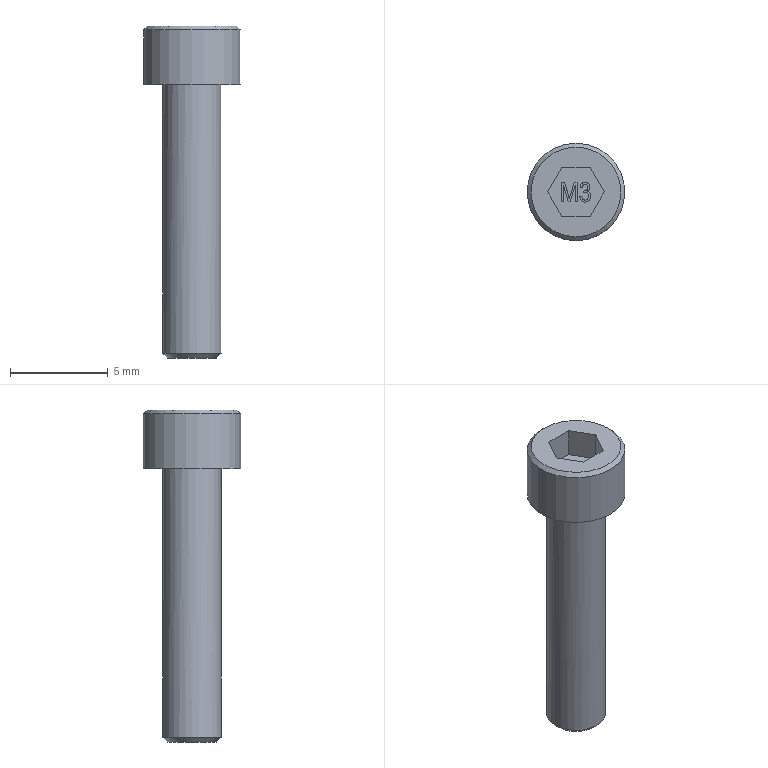Part | STEP file | EM10301400 | 1 solid | 37 faces | box 5 x 5 x 17 mm | volume 149.174 mm3 | plane 26 | other 7 | cylinder 2 | cone 2 | commonest cylinder face diameters 3 x1 5 x1